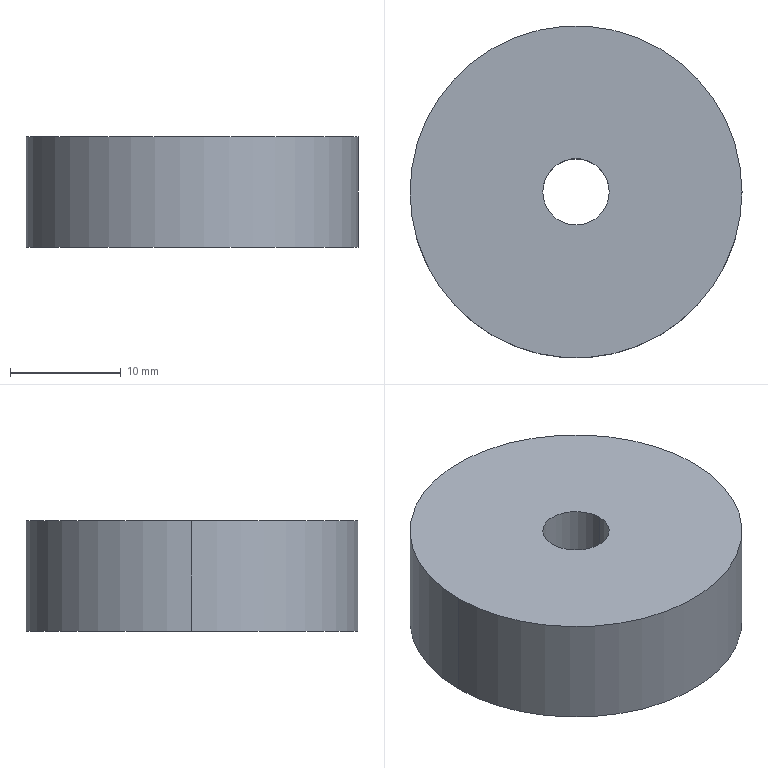Part | STEP file | Small locating block | 1 solid | 6 faces | box 30 x 30 x 10 mm | volume 6786 mm3 | cylinder 4 | plane 2 | commonest cylinder face diameters 6 x2 30 x2
STEP:
#1=CARTESIAN_POINT('',(0.,0.,0.));
#2=DIRECTION('',(0.,0.,1.));
#3=DIRECTION('',(1.,0.,0.));
#4=AXIS2_PLACEMENT_3D('',#1,#2,#3);
#5=CARTESIAN_POINT('',(-3.,0.,10.));
#6=VERTEX_POINT('',#5);
#7=CARTESIAN_POINT('',(-3.,0.,0.));
#8=VERTEX_POINT('',#7);
#9=CARTESIAN_POINT('',(-3.,0.,10.));
#10=DIRECTION('',(0.,0.,-1.));
#11=VECTOR('',#10,1.);
#12=LINE('',#9,#11);
#13=CARTESIAN_POINT('',(0.,0.,10.));
#14=DIRECTION('',(0.,0.,-1.));
#15=DIRECTION('',(-1.,0.,0.));
#16=AXIS2_PLACEMENT_3D('',#13,#14,#15);
#17=CYLINDRICAL_SURFACE('',#16,3.);
#18=CARTESIAN_POINT('',(6.283,0.));
#19=DIRECTION('',(0.,1.));
#20=VECTOR('',#19,1.);
#21=LINE('',#18,#20);
#22=(GEOMETRIC_REPRESENTATION_CONTEXT(2)PARAMETRIC_REPRESENTATION_CONTEXT()REPRESENTATION_CONTEXT('',''));
#23=DEFINITIONAL_REPRESENTATION('',(#21),#22);
#24=PCURVE('',#17,#23);
#25=CARTESIAN_POINT('',(0.,0.,10.));
#26=DIRECTION('',(0.,0.,-1.));
#27=DIRECTION('',(-1.,0.,0.));
#28=AXIS2_PLACEMENT_3D('',#25,#26,#27);
#29=CYLINDRICAL_SURFACE('',#28,3.);
#30=CARTESIAN_POINT('',(0.,0.));
#31=DIRECTION('',(0.,1.));
#32=VECTOR('',#31,1.);
#33=LINE('',#30,#32);
#34=(GEOMETRIC_REPRESENTATION_CONTEXT(2)PARAMETRIC_REPRESENTATION_CONTEXT()REPRESENTATION_CONTEXT('',''));
#35=DEFINITIONAL_REPRESENTATION('',(#33),#34);
#36=PCURVE('',#29,#35);
#37=SURFACE_CURVE('',#12,(#24,#36),.PCURVE_S1.);
#38=EDGE_CURVE('',#6,#8,#37,.T.);
#39=ORIENTED_EDGE('',*,*,#38,.T.);
#40=CARTESIAN_POINT('',(3.,0.,0.));
#41=VERTEX_POINT('',#40);
#42=CARTESIAN_POINT('',(0.,0.,0.));
#43=DIRECTION('',(0.,0.,1.));
#44=DIRECTION('',(1.,0.,0.));
#45=AXIS2_PLACEMENT_3D('',#42,#43,#44);
#46=CIRCLE('',#45,3.);
#47=CARTESIAN_POINT('',(9.425,10.));
#48=DIRECTION('',(-1.,0.));
#49=VECTOR('',#48,1.);
#50=LINE('',#47,#49);
#51=(GEOMETRIC_REPRESENTATION_CONTEXT(2)PARAMETRIC_REPRESENTATION_CONTEXT()REPRESENTATION_CONTEXT('',''));
#52=DEFINITIONAL_REPRESENTATION('',(#50),#51);
#53=PCURVE('',#17,#52);
#54=CARTESIAN_POINT('',(0.,0.,0.));
#55=DIRECTION('',(0.,0.,1.));
#56=DIRECTION('',(1.,0.,0.));
#57=AXIS2_PLACEMENT_3D('',#54,#55,#56);
#58=PLANE('',#57);
#59=CARTESIAN_POINT('',(0.,0.));
#60=DIRECTION('',(1.,0.));
#61=AXIS2_PLACEMENT_2D('',#59,#60);
#62=CIRCLE('',#61,3.);
#63=(GEOMETRIC_REPRESENTATION_CONTEXT(2)PARAMETRIC_REPRESENTATION_CONTEXT()REPRESENTATION_CONTEXT('',''));
#64=DEFINITIONAL_REPRESENTATION('',(#62),#63);
#65=PCURVE('',#58,#64);
#66=SURFACE_CURVE('',#46,(#53,#65),.PCURVE_S1.);
#67=EDGE_CURVE('',#8,#41,#66,.T.);
#68=ORIENTED_EDGE('',*,*,#67,.T.);
#69=CARTESIAN_POINT('',(3.,0.,10.));
#70=VERTEX_POINT('',#69);
#71=CARTESIAN_POINT('',(3.,0.,10.));
#72=DIRECTION('',(0.,0.,-1.));
#73=VECTOR('',#72,1.);
#74=LINE('',#71,#73);
#75=CARTESIAN_POINT('',(3.142,0.));
#76=DIRECTION('',(0.,1.));
#77=VECTOR('',#76,1.);
#78=LINE('',#75,#77);
#79=(GEOMETRIC_REPRESENTATION_CONTEXT(2)PARAMETRIC_REPRESENTATION_CONTEXT()REPRESENTATION_CONTEXT('',''));
#80=DEFINITIONAL_REPRESENTATION('',(#78),#79);
#81=PCURVE('',#17,#80);
#82=CARTESIAN_POINT('',(3.142,0.));
#83=DIRECTION('',(0.,1.));
#84=VECTOR('',#83,1.);
#85=LINE('',#82,#84);
#86=(GEOMETRIC_REPRESENTATION_CONTEXT(2)PARAMETRIC_REPRESENTATION_CONTEXT()REPRESENTATION_CONTEXT('',''));
#87=DEFINITIONAL_REPRESENTATION('',(#85),#86);
#88=PCURVE('',#29,#87);
#89=SURFACE_CURVE('',#74,(#81,#88),.PCURVE_S1.);
#90=EDGE_CURVE('',#70,#41,#89,.T.);
#91=ORIENTED_EDGE('',*,*,#90,.F.);
#92=CARTESIAN_POINT('',(0.,0.,10.));
#93=DIRECTION('',(0.,0.,1.));
#94=DIRECTION('',(1.,0.,0.));
#95=AXIS2_PLACEMENT_3D('',#92,#93,#94);
#96=CIRCLE('',#95,3.);
#97=CARTESIAN_POINT('',(9.425,0.));
#98=DIRECTION('',(-1.,0.));
#99=VECTOR('',#98,1.);
#100=LINE('',#97,#99);
#101=(GEOMETRIC_REPRESENTATION_CONTEXT(2)PARAMETRIC_REPRESENTATION_CONTEXT()REPRESENTATION_CONTEXT('',''));
#102=DEFINITIONAL_REPRESENTATION('',(#100),#101);
#103=PCURVE('',#17,#102);
#104=CARTESIAN_POINT('',(0.,0.,10.));
#105=DIRECTION('',(0.,0.,1.));
#106=DIRECTION('',(1.,0.,0.));
#107=AXIS2_PLACEMENT_3D('',#104,#105,#106);
#108=PLANE('',#107);
#109=CARTESIAN_POINT('',(0.,0.));
#110=DIRECTION('',(1.,0.));
#111=AXIS2_PLACEMENT_2D('',#109,#110);
#112=CIRCLE('',#111,3.);
#113=(GEOMETRIC_REPRESENTATION_CONTEXT(2)PARAMETRIC_REPRESENTATION_CONTEXT()REPRESENTATION_CONTEXT('',''));
#114=DEFINITIONAL_REPRESENTATION('',(#112),#113);
#115=PCURVE('',#108,#114);
#116=SURFACE_CURVE('',#96,(#103,#115),.PCURVE_S1.);
#117=EDGE_CURVE('',#6,#70,#116,.T.);
#118=ORIENTED_EDGE('',*,*,#117,.F.);
#119=EDGE_LOOP('',(#39,#68,#91,#118));
#120=FACE_BOUND('',#119,.F.);
#121=ADVANCED_FACE('',(#120),#17,.F.);
#122=CARTESIAN_POINT('',(15.,0.,10.));
#123=VERTEX_POINT('',#122);
#124=CARTESIAN_POINT('',(-15.,0.,10.));
#125=VERTEX_POINT('',#124);
#126=CARTESIAN_POINT('',(0.,0.,10.));
#127=DIRECTION('',(0.,0.,1.));
#128=DIRECTION('',(1.,0.,0.));
#129=AXIS2_PLACEMENT_3D('',#126,#127,#128);
#130=CIRCLE('',#129,15.);
#131=CARTESIAN_POINT('',(0.,0.,10.));
#132=DIRECTION('',(0.,0.,-1.));
#133=DIRECTION('',(-1.,0.,0.));
#134=AXIS2_PLACEMENT_3D('',#131,#132,#133);
#135=CYLINDRICAL_SURFACE('',#134,15.);
#136=CARTESIAN_POINT('',(3.142,0.));
#137=DIRECTION('',(-1.,0.));
#138=VECTOR('',#137,1.);
#139=LINE('',#136,#138);
#140=(GEOMETRIC_REPRESENTATION_CONTEXT(2)PARAMETRIC_REPRESENTATION_CONTEXT()REPRESENTATION_CONTEXT('',''));
#141=DEFINITIONAL_REPRESENTATION('',(#139),#140);
#142=PCURVE('',#135,#141);
#143=CARTESIAN_POINT('',(0.,0.));
#144=DIRECTION('',(1.,0.));
#145=AXIS2_PLACEMENT_2D('',#143,#144);
#146=CIRCLE('',#145,15.);
#147=(GEOMETRIC_REPRESENTATION_CONTEXT(2)PARAMETRIC_REPRESENTATION_CONTEXT()REPRESENTATION_CONTEXT('',''));
#148=DEFINITIONAL_REPRESENTATION('',(#146),#147);
#149=PCURVE('',#108,#148);
#150=SURFACE_CURVE('',#130,(#142,#149),.PCURVE_S1.);
#151=EDGE_CURVE('',#123,#125,#150,.T.);
#152=ORIENTED_EDGE('',*,*,#151,.F.);
#153=CARTESIAN_POINT('',(15.,0.,0.));
#154=VERTEX_POINT('',#153);
#155=CARTESIAN_POINT('',(15.,0.,10.));
#156=DIRECTION('',(0.,0.,-1.));
#157=VECTOR('',#156,1.);
#158=LINE('',#155,#157);
#159=CARTESIAN_POINT('',(3.142,0.));
#160=DIRECTION('',(0.,1.));
#161=VECTOR('',#160,1.);
#162=LINE('',#159,#161);
#163=(GEOMETRIC_REPRESENTATION_CONTEXT(2)PARAMETRIC_REPRESENTATION_CONTEXT()REPRESENTATION_CONTEXT('',''));
#164=DEFINITIONAL_REPRESENTATION('',(#162),#163);
#165=PCURVE('',#135,#164);
#166=CARTESIAN_POINT('',(0.,0.,10.));
#167=DIRECTION('',(0.,0.,-1.));
#168=DIRECTION('',(-1.,0.,0.));
#169=AXIS2_PLACEMENT_3D('',#166,#167,#168);
#170=CYLINDRICAL_SURFACE('',#169,15.);
#171=CARTESIAN_POINT('',(3.142,0.));
#172=DIRECTION('',(0.,1.));
#173=VECTOR('',#172,1.);
#174=LINE('',#171,#173);
#175=(GEOMETRIC_REPRESENTATION_CONTEXT(2)PARAMETRIC_REPRESENTATION_CONTEXT()REPRESENTATION_CONTEXT('',''));
#176=DEFINITIONAL_REPRESENTATION('',(#174),#175);
#177=PCURVE('',#170,#176);
#178=SURFACE_CURVE('',#158,(#165,#177),.PCURVE_S1.);
#179=EDGE_CURVE('',#123,#154,#178,.T.);
#180=ORIENTED_EDGE('',*,*,#179,.T.);
#181=CARTESIAN_POINT('',(-15.,0.,0.));
#182=VERTEX_POINT('',#181);
#183=CARTESIAN_POINT('',(0.,0.,0.));
#184=DIRECTION('',(0.,0.,1.));
#185=DIRECTION('',(1.,0.,0.));
#186=AXIS2_PLACEMENT_3D('',#183,#184,#185);
#187=CIRCLE('',#186,15.);
#188=CARTESIAN_POINT('',(3.142,10.));
#189=DIRECTION('',(-1.,0.));
#190=VECTOR('',#189,1.);
#191=LINE('',#188,#190);
#192=(GEOMETRIC_REPRESENTATION_CONTEXT(2)PARAMETRIC_REPRESENTATION_CONTEXT()REPRESENTATION_CONTEXT('',''));
#193=DEFINITIONAL_REPRESENTATION('',(#191),#192);
#194=PCURVE('',#135,#193);
#195=CARTESIAN_POINT('',(0.,0.));
#196=DIRECTION('',(1.,0.));
#197=AXIS2_PLACEMENT_2D('',#195,#196);
#198=CIRCLE('',#197,15.);
#199=(GEOMETRIC_REPRESENTATION_CONTEXT(2)PARAMETRIC_REPRESENTATION_CONTEXT()REPRESENTATION_CONTEXT('',''));
#200=DEFINITIONAL_REPRESENTATION('',(#198),#199);
#201=PCURVE('',#58,#200);
#202=SURFACE_CURVE('',#187,(#194,#201),.PCURVE_S1.);
#203=EDGE_CURVE('',#154,#182,#202,.T.);
#204=ORIENTED_EDGE('',*,*,#203,.T.);
#205=CARTESIAN_POINT('',(-15.,0.,10.));
#206=DIRECTION('',(0.,0.,-1.));
#207=VECTOR('',#206,1.);
#208=LINE('',#205,#207);
#209=CARTESIAN_POINT('',(0.,0.));
#210=DIRECTION('',(0.,1.));
#211=VECTOR('',#210,1.);
#212=LINE('',#209,#211);
#213=(GEOMETRIC_REPRESENTATION_CONTEXT(2)PARAMETRIC_REPRESENTATION_CONTEXT()REPRESENTATION_CONTEXT('',''));
#214=DEFINITIONAL_REPRESENTATION('',(#212),#213);
#215=PCURVE('',#135,#214);
#216=CARTESIAN_POINT('',(6.283,0.));
#217=DIRECTION('',(0.,1.));
#218=VECTOR('',#217,1.);
#219=LINE('',#216,#218);
#220=(GEOMETRIC_REPRESENTATION_CONTEXT(2)PARAMETRIC_REPRESENTATION_CONTEXT()REPRESENTATION_CONTEXT('',''));
#221=DEFINITIONAL_REPRESENTATION('',(#219),#220);
#222=PCURVE('',#170,#221);
#223=SURFACE_CURVE('',#208,(#215,#222),.PCURVE_S1.);
#224=EDGE_CURVE('',#125,#182,#223,.T.);
#225=ORIENTED_EDGE('',*,*,#224,.F.);
#226=EDGE_LOOP('',(#152,#180,#204,#225));
#227=FACE_BOUND('',#226,.T.);
#228=ADVANCED_FACE('',(#227),#135,.T.);
#229=CARTESIAN_POINT('',(0.,0.,10.));
#230=DIRECTION('',(0.,0.,1.));
#231=DIRECTION('',(1.,0.,0.));
#232=AXIS2_PLACEMENT_3D('',#229,#230,#231);
#233=CIRCLE('',#232,15.);
#234=CARTESIAN_POINT('',(0.,0.));
#235=DIRECTION('',(1.,0.));
#236=AXIS2_PLACEMENT_2D('',#234,#235);
#237=CIRCLE('',#236,15.);
#238=(GEOMETRIC_REPRESENTATION_CONTEXT(2)PARAMETRIC_REPRESENTATION_CONTEXT()REPRESENTATION_CONTEXT('',''));
#239=DEFINITIONAL_REPRESENTATION('',(#237),#238);
#240=PCURVE('',#108,#239);
#241=CARTESIAN_POINT('',(9.425,0.));
#242=DIRECTION('',(-1.,0.));
#243=VECTOR('',#242,1.);
#244=LINE('',#241,#243);
#245=(GEOMETRIC_REPRESENTATION_CONTEXT(2)PARAMETRIC_REPRESENTATION_CONTEXT()REPRESENTATION_CONTEXT('',''));
#246=DEFINITIONAL_REPRESENTATION('',(#244),#245);
#247=PCURVE('',#170,#246);
#248=SURFACE_CURVE('',#233,(#240,#247),.PCURVE_S1.);
#249=EDGE_CURVE('',#125,#123,#248,.T.);
#250=ORIENTED_EDGE('',*,*,#249,.T.);
#251=ORIENTED_EDGE('',*,*,#151,.T.);
#252=EDGE_LOOP('',(#250,#251));
#253=FACE_BOUND('',#252,.T.);
#254=ORIENTED_EDGE('',*,*,#117,.F.);
#255=CARTESIAN_POINT('',(0.,0.,10.));
#256=DIRECTION('',(0.,0.,1.));
#257=DIRECTION('',(1.,0.,0.));
#258=AXIS2_PLACEMENT_3D('',#255,#256,#257);
#259=CIRCLE('',#258,3.);
#260=CARTESIAN_POINT('',(0.,0.));
#261=DIRECTION('',(1.,0.));
#262=AXIS2_PLACEMENT_2D('',#260,#261);
#263=CIRCLE('',#262,3.);
#264=(GEOMETRIC_REPRESENTATION_CONTEXT(2)PARAMETRIC_REPRESENTATION_CONTEXT()REPRESENTATION_CONTEXT('',''));
#265=DEFINITIONAL_REPRESENTATION('',(#263),#264);
#266=PCURVE('',#108,#265);
#267=CARTESIAN_POINT('',(3.142,0.));
#268=DIRECTION('',(-1.,0.));
#269=VECTOR('',#268,1.);
#270=LINE('',#267,#269);
#271=(GEOMETRIC_REPRESENTATION_CONTEXT(2)PARAMETRIC_REPRESENTATION_CONTEXT()REPRESENTATION_CONTEXT('',''));
#272=DEFINITIONAL_REPRESENTATION('',(#270),#271);
#273=PCURVE('',#29,#272);
#274=SURFACE_CURVE('',#259,(#266,#273),.PCURVE_S1.);
#275=EDGE_CURVE('',#70,#6,#274,.T.);
#276=ORIENTED_EDGE('',*,*,#275,.F.);
#277=EDGE_LOOP('',(#254,#276));
#278=FACE_BOUND('',#277,.T.);
#279=ADVANCED_FACE('',(#253,#278),#108,.T.);
#280=CARTESIAN_POINT('',(0.,0.,0.));
#281=DIRECTION('',(0.,0.,1.));
#282=DIRECTION('',(1.,0.,0.));
#283=AXIS2_PLACEMENT_3D('',#280,#281,#282);
#284=CIRCLE('',#283,15.);
#285=CARTESIAN_POINT('',(0.,0.));
#286=DIRECTION('',(1.,0.));
#287=AXIS2_PLACEMENT_2D('',#285,#286);
#288=CIRCLE('',#287,15.);
#289=(GEOMETRIC_REPRESENTATION_CONTEXT(2)PARAMETRIC_REPRESENTATION_CONTEXT()REPRESENTATION_CONTEXT('',''));
#290=DEFINITIONAL_REPRESENTATION('',(#288),#289);
#291=PCURVE('',#58,#290);
#292=CARTESIAN_POINT('',(9.425,10.));
#293=DIRECTION('',(-1.,0.));
#294=VECTOR('',#293,1.);
#295=LINE('',#292,#294);
#296=(GEOMETRIC_REPRESENTATION_CONTEXT(2)PARAMETRIC_REPRESENTATION_CONTEXT()REPRESENTATION_CONTEXT('',''));
#297=DEFINITIONAL_REPRESENTATION('',(#295),#296);
#298=PCURVE('',#170,#297);
#299=SURFACE_CURVE('',#284,(#291,#298),.PCURVE_S1.);
#300=EDGE_CURVE('',#182,#154,#299,.T.);
#301=ORIENTED_EDGE('',*,*,#300,.F.);
#302=ORIENTED_EDGE('',*,*,#203,.F.);
#303=EDGE_LOOP('',(#301,#302));
#304=FACE_BOUND('',#303,.T.);
#305=ORIENTED_EDGE('',*,*,#67,.T.);
#306=CARTESIAN_POINT('',(0.,0.,0.));
#307=DIRECTION('',(0.,0.,1.));
#308=DIRECTION('',(1.,0.,0.));
#309=AXIS2_PLACEMENT_3D('',#306,#307,#308);
#310=CIRCLE('',#309,3.);
#311=CARTESIAN_POINT('',(0.,0.));
#312=DIRECTION('',(1.,0.));
#313=AXIS2_PLACEMENT_2D('',#311,#312);
#314=CIRCLE('',#313,3.);
#315=(GEOMETRIC_REPRESENTATION_CONTEXT(2)PARAMETRIC_REPRESENTATION_CONTEXT()REPRESENTATION_CONTEXT('',''));
#316=DEFINITIONAL_REPRESENTATION('',(#314),#315);
#317=PCURVE('',#58,#316);
#318=CARTESIAN_POINT('',(3.142,10.));
#319=DIRECTION('',(-1.,0.));
#320=VECTOR('',#319,1.);
#321=LINE('',#318,#320);
#322=(GEOMETRIC_REPRESENTATION_CONTEXT(2)PARAMETRIC_REPRESENTATION_CONTEXT()REPRESENTATION_CONTEXT('',''));
#323=DEFINITIONAL_REPRESENTATION('',(#321),#322);
#324=PCURVE('',#29,#323);
#325=SURFACE_CURVE('',#310,(#317,#324),.PCURVE_S1.);
#326=EDGE_CURVE('',#41,#8,#325,.T.);
#327=ORIENTED_EDGE('',*,*,#326,.T.);
#328=EDGE_LOOP('',(#305,#327));
#329=FACE_BOUND('',#328,.T.);
#330=ADVANCED_FACE('',(#304,#329),#58,.F.);
#331=ORIENTED_EDGE('',*,*,#179,.F.);
#332=ORIENTED_EDGE('',*,*,#249,.F.);
#333=ORIENTED_EDGE('',*,*,#224,.T.);
#334=ORIENTED_EDGE('',*,*,#300,.T.);
#335=EDGE_LOOP('',(#331,#332,#333,#334));
#336=FACE_BOUND('',#335,.T.);
#337=ADVANCED_FACE('',(#336),#170,.T.);
#338=ORIENTED_EDGE('',*,*,#326,.T.);
#339=ORIENTED_EDGE('',*,*,#38,.F.);
#340=ORIENTED_EDGE('',*,*,#275,.F.);
#341=ORIENTED_EDGE('',*,*,#90,.T.);
#342=EDGE_LOOP('',(#338,#339,#340,#341));
#343=FACE_BOUND('',#342,.F.);
#344=ADVANCED_FACE('',(#343),#29,.F.);
#345=CLOSED_SHELL('',(#121,#228,#279,#330,#337,#344));
#346=MANIFOLD_SOLID_BREP('',#345);
#347=(LENGTH_UNIT()NAMED_UNIT(*)SI_UNIT(.MILLI.,.METRE.));
#348=UNCERTAINTY_MEASURE_WITH_UNIT(LENGTH_MEASURE(0.0000001),#347,'','');
#349=(NAMED_UNIT(*)PLANE_ANGLE_UNIT()SI_UNIT($,.RADIAN.));
#350=(NAMED_UNIT(*)SI_UNIT($,.STERADIAN.)SOLID_ANGLE_UNIT());
#351=(GEOMETRIC_REPRESENTATION_CONTEXT(3)GLOBAL_UNCERTAINTY_ASSIGNED_CONTEXT((#348))GLOBAL_UNIT_ASSIGNED_CONTEXT((#347,#349,#350))REPRESENTATION_CONTEXT('',''));
#352=ADVANCED_BREP_SHAPE_REPRESENTATION('',(#4,#346),#351);